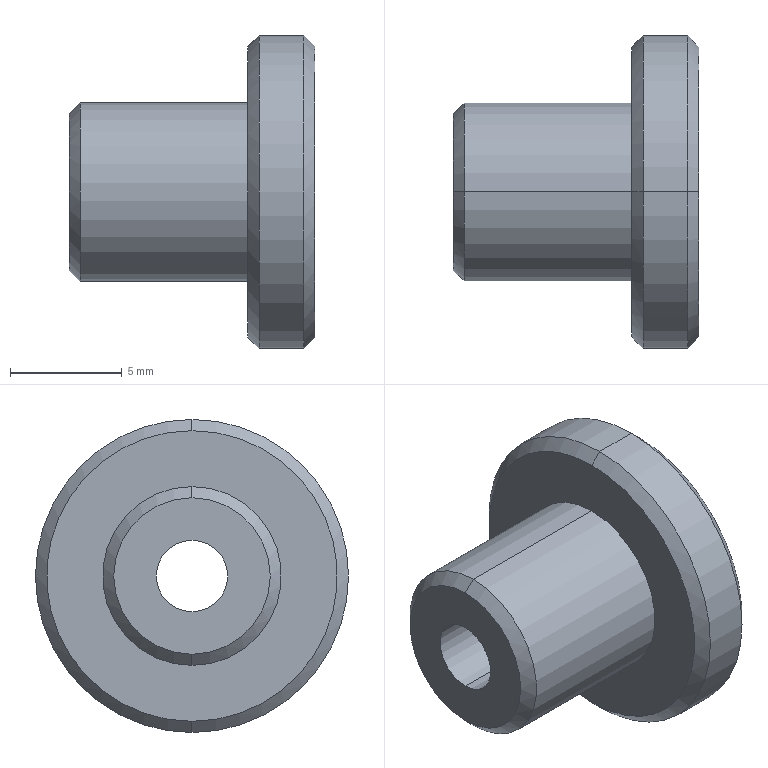Part | SolidWorks | features Chamfer 1, Revolution 1 | 1 solid | 17 faces | box 11 x 14 x 14 mm | volume 760.339 mm3 | cone 8 | cylinder 6 | plane 3 | commonest cylinder face diameters 3.2 x2 8 x2 14 x2
STEP:
#1=CARTESIAN_POINT('',(17.,26.043,1.6));
#2=VERTEX_POINT('',#1);
#3=CARTESIAN_POINT('',(17.,26.043,-1.6));
#4=VERTEX_POINT('',#3);
#5=CARTESIAN_POINT('',(17.,26.043,0.));
#6=DIRECTION('',(1.,0.,0.));
#7=DIRECTION('',(0.,0.,-1.));
#8=AXIS2_PLACEMENT_3D('',#5,#6,#7);
#9=CIRCLE('',#8,1.6);
#10=EDGE_CURVE('',#2,#4,#9,.T.);
#11=ORIENTED_EDGE('',*,*,#10,.F.);
#12=CARTESIAN_POINT('',(17.5,26.043,2.1));
#13=VERTEX_POINT('',#12);
#14=CARTESIAN_POINT('',(17.,26.043,1.6));
#15=DIRECTION('',(0.7071,0.,0.7071));
#16=VECTOR('',#15,1000.);
#17=LINE('',#14,#16);
#18=EDGE_CURVE('',#2,#13,#17,.T.);
#19=ORIENTED_EDGE('',*,*,#18,.T.);
#20=CARTESIAN_POINT('',(17.5,26.043,-2.1));
#21=VERTEX_POINT('',#20);
#22=CARTESIAN_POINT('',(17.5,26.043,0.));
#23=DIRECTION('',(-1.,0.,0.));
#24=DIRECTION('',(0.,0.,-1.));
#25=AXIS2_PLACEMENT_3D('',#22,#23,#24);
#26=CIRCLE('',#25,2.1);
#27=EDGE_CURVE('',#21,#13,#26,.T.);
#28=ORIENTED_EDGE('',*,*,#27,.F.);
#29=CARTESIAN_POINT('',(17.,26.043,-1.6));
#30=DIRECTION('',(0.7071,0.,-0.7071));
#31=VECTOR('',#30,1000.);
#32=LINE('',#29,#31);
#33=EDGE_CURVE('',#4,#21,#32,.T.);
#34=ORIENTED_EDGE('',*,*,#33,.F.);
#35=EDGE_LOOP('',(#11,#19,#28,#34));
#36=FACE_OUTER_BOUND('',#35,.T.);
#37=CARTESIAN_POINT('',(17.,26.043,0.));
#38=DIRECTION('',(1.,0.,0.));
#39=DIRECTION('',(0.,0.,-1.));
#40=AXIS2_PLACEMENT_3D('',#37,#38,#39);
#41=CONICAL_SURFACE('',#40,1.6,0.7854);
#42=ADVANCED_FACE('',(#36),#41,.F.);
#43=CARTESIAN_POINT('',(6.5,26.043,3.5));
#44=VERTEX_POINT('',#43);
#45=CARTESIAN_POINT('',(6.5,26.043,-3.5));
#46=VERTEX_POINT('',#45);
#47=CARTESIAN_POINT('',(6.5,26.043,0.));
#48=DIRECTION('',(-1.,0.,0.));
#49=DIRECTION('',(0.,0.,1.));
#50=AXIS2_PLACEMENT_3D('',#47,#48,#49);
#51=CIRCLE('',#50,3.5);
#52=EDGE_CURVE('',#44,#46,#51,.T.);
#53=ORIENTED_EDGE('',*,*,#52,.F.);
#54=CARTESIAN_POINT('',(7.,26.043,4.));
#55=VERTEX_POINT('',#54);
#56=CARTESIAN_POINT('',(7.,26.043,4.));
#57=DIRECTION('',(0.7071,0.,0.7071));
#58=VECTOR('',#57,1000.);
#59=LINE('',#56,#58);
#60=EDGE_CURVE('',#44,#55,#59,.T.);
#61=ORIENTED_EDGE('',*,*,#60,.T.);
#62=CARTESIAN_POINT('',(7.,26.043,-4.));
#63=VERTEX_POINT('',#62);
#64=CARTESIAN_POINT('',(7.,26.043,0.));
#65=DIRECTION('',(1.,0.,0.));
#66=DIRECTION('',(0.,0.,1.));
#67=AXIS2_PLACEMENT_3D('',#64,#65,#66);
#68=CIRCLE('',#67,4.);
#69=EDGE_CURVE('',#63,#55,#68,.T.);
#70=ORIENTED_EDGE('',*,*,#69,.F.);
#71=CARTESIAN_POINT('',(7.,26.043,-4.));
#72=DIRECTION('',(0.7071,0.,-0.7071));
#73=VECTOR('',#72,1000.);
#74=LINE('',#71,#73);
#75=EDGE_CURVE('',#46,#63,#74,.T.);
#76=ORIENTED_EDGE('',*,*,#75,.F.);
#77=EDGE_LOOP('',(#53,#61,#70,#76));
#78=FACE_OUTER_BOUND('',#77,.T.);
#79=CARTESIAN_POINT('',(7.,26.043,0.));
#80=DIRECTION('',(1.,0.,0.));
#81=DIRECTION('',(0.,0.,-1.));
#82=AXIS2_PLACEMENT_3D('',#79,#80,#81);
#83=CONICAL_SURFACE('',#82,4.,0.7854);
#84=ADVANCED_FACE('',(#78),#83,.T.);
#85=CARTESIAN_POINT('',(17.5,26.043,-6.5));
#86=VERTEX_POINT('',#85);
#87=CARTESIAN_POINT('',(17.5,26.043,6.5));
#88=VERTEX_POINT('',#87);
#89=CARTESIAN_POINT('',(17.5,26.043,0.));
#90=DIRECTION('',(1.,0.,0.));
#91=DIRECTION('',(0.,0.,-1.));
#92=AXIS2_PLACEMENT_3D('',#89,#90,#91);
#93=CIRCLE('',#92,6.5);
#94=EDGE_CURVE('',#86,#88,#93,.T.);
#95=ORIENTED_EDGE('',*,*,#94,.F.);
#96=CARTESIAN_POINT('',(17.,26.043,-7.));
#97=VERTEX_POINT('',#96);
#98=CARTESIAN_POINT('',(17.5,26.043,-6.5));
#99=DIRECTION('',(-0.7071,0.,-0.7071));
#100=VECTOR('',#99,1000.);
#101=LINE('',#98,#100);
#102=EDGE_CURVE('',#86,#97,#101,.T.);
#103=ORIENTED_EDGE('',*,*,#102,.T.);
#104=CARTESIAN_POINT('',(17.,26.043,7.));
#105=VERTEX_POINT('',#104);
#106=CARTESIAN_POINT('',(17.,26.043,0.));
#107=DIRECTION('',(-1.,0.,0.));
#108=DIRECTION('',(0.,0.,-1.));
#109=AXIS2_PLACEMENT_3D('',#106,#107,#108);
#110=CIRCLE('',#109,7.);
#111=EDGE_CURVE('',#105,#97,#110,.T.);
#112=ORIENTED_EDGE('',*,*,#111,.F.);
#113=CARTESIAN_POINT('',(17.5,26.043,6.5));
#114=DIRECTION('',(-0.7071,0.,0.7071));
#115=VECTOR('',#114,1000.);
#116=LINE('',#113,#115);
#117=EDGE_CURVE('',#88,#105,#116,.T.);
#118=ORIENTED_EDGE('',*,*,#117,.F.);
#119=EDGE_LOOP('',(#95,#103,#112,#118));
#120=FACE_OUTER_BOUND('',#119,.T.);
#121=CARTESIAN_POINT('',(17.5,26.043,0.));
#122=DIRECTION('',(-1.,0.,0.));
#123=DIRECTION('',(0.,0.,1.));
#124=AXIS2_PLACEMENT_3D('',#121,#122,#123);
#125=CONICAL_SURFACE('',#124,6.5,0.7854);
#126=ADVANCED_FACE('',(#120),#125,.T.);
#127=CARTESIAN_POINT('',(14.5,26.043,6.5));
#128=VERTEX_POINT('',#127);
#129=CARTESIAN_POINT('',(14.5,26.043,-6.5));
#130=VERTEX_POINT('',#129);
#131=CARTESIAN_POINT('',(14.5,26.043,0.));
#132=DIRECTION('',(-1.,0.,0.));
#133=DIRECTION('',(0.,0.,1.));
#134=AXIS2_PLACEMENT_3D('',#131,#132,#133);
#135=CIRCLE('',#134,6.5);
#136=EDGE_CURVE('',#128,#130,#135,.T.);
#137=ORIENTED_EDGE('',*,*,#136,.F.);
#138=CARTESIAN_POINT('',(15.,26.043,7.));
#139=VERTEX_POINT('',#138);
#140=CARTESIAN_POINT('',(15.,26.043,7.));
#141=DIRECTION('',(0.7071,0.,0.7071));
#142=VECTOR('',#141,1000.);
#143=LINE('',#140,#142);
#144=EDGE_CURVE('',#128,#139,#143,.T.);
#145=ORIENTED_EDGE('',*,*,#144,.T.);
#146=CARTESIAN_POINT('',(15.,26.043,-7.));
#147=VERTEX_POINT('',#146);
#148=CARTESIAN_POINT('',(15.,26.043,0.));
#149=DIRECTION('',(1.,0.,0.));
#150=DIRECTION('',(0.,0.,1.));
#151=AXIS2_PLACEMENT_3D('',#148,#149,#150);
#152=CIRCLE('',#151,7.);
#153=EDGE_CURVE('',#147,#139,#152,.T.);
#154=ORIENTED_EDGE('',*,*,#153,.F.);
#155=CARTESIAN_POINT('',(15.,26.043,-7.));
#156=DIRECTION('',(0.7071,0.,-0.7071));
#157=VECTOR('',#156,1000.);
#158=LINE('',#155,#157);
#159=EDGE_CURVE('',#130,#147,#158,.T.);
#160=ORIENTED_EDGE('',*,*,#159,.F.);
#161=EDGE_LOOP('',(#137,#145,#154,#160));
#162=FACE_OUTER_BOUND('',#161,.T.);
#163=CARTESIAN_POINT('',(15.,26.043,0.));
#164=DIRECTION('',(1.,0.,0.));
#165=DIRECTION('',(0.,0.,-1.));
#166=AXIS2_PLACEMENT_3D('',#163,#164,#165);
#167=CONICAL_SURFACE('',#166,7.,0.7854);
#168=ADVANCED_FACE('',(#162),#167,.T.);
#169=ORIENTED_EDGE('',*,*,#153,.T.);
#170=CARTESIAN_POINT('',(17.5,26.043,7.));
#171=DIRECTION('',(1.,0.,0.));
#172=VECTOR('',#171,1000.);
#173=LINE('',#170,#172);
#174=EDGE_CURVE('',#139,#105,#173,.T.);
#175=ORIENTED_EDGE('',*,*,#174,.T.);
#176=ORIENTED_EDGE('',*,*,#111,.T.);
#177=CARTESIAN_POINT('',(17.5,26.043,-7.));
#178=DIRECTION('',(1.,0.,0.));
#179=VECTOR('',#178,1000.);
#180=LINE('',#177,#179);
#181=EDGE_CURVE('',#147,#97,#180,.T.);
#182=ORIENTED_EDGE('',*,*,#181,.F.);
#183=EDGE_LOOP('',(#169,#175,#176,#182));
#184=FACE_OUTER_BOUND('',#183,.T.);
#185=CARTESIAN_POINT('',(17.5,26.043,0.));
#186=DIRECTION('',(1.,0.,0.));
#187=DIRECTION('',(0.,0.,-1.));
#188=AXIS2_PLACEMENT_3D('',#185,#186,#187);
#189=CYLINDRICAL_SURFACE('',#188,7.);
#190=ADVANCED_FACE('',(#184),#189,.T.);
#191=ORIENTED_EDGE('',*,*,#69,.T.);
#192=CARTESIAN_POINT('',(14.5,26.043,4.));
#193=VERTEX_POINT('',#192);
#194=CARTESIAN_POINT('',(17.5,26.043,4.));
#195=DIRECTION('',(1.,0.,0.));
#196=VECTOR('',#195,1000.);
#197=LINE('',#194,#196);
#198=EDGE_CURVE('',#55,#193,#197,.T.);
#199=ORIENTED_EDGE('',*,*,#198,.T.);
#200=CARTESIAN_POINT('',(14.5,26.043,-4.));
#201=VERTEX_POINT('',#200);
#202=CARTESIAN_POINT('',(14.5,26.043,0.));
#203=DIRECTION('',(1.,0.,0.));
#204=DIRECTION('',(0.,0.,-1.));
#205=AXIS2_PLACEMENT_3D('',#202,#203,#204);
#206=CIRCLE('',#205,4.);
#207=EDGE_CURVE('',#201,#193,#206,.T.);
#208=ORIENTED_EDGE('',*,*,#207,.F.);
#209=CARTESIAN_POINT('',(17.5,26.043,-4.));
#210=DIRECTION('',(1.,0.,0.));
#211=VECTOR('',#210,1000.);
#212=LINE('',#209,#211);
#213=EDGE_CURVE('',#63,#201,#212,.T.);
#214=ORIENTED_EDGE('',*,*,#213,.F.);
#215=EDGE_LOOP('',(#191,#199,#208,#214));
#216=FACE_OUTER_BOUND('',#215,.T.);
#217=CARTESIAN_POINT('',(17.5,26.043,0.));
#218=DIRECTION('',(1.,0.,0.));
#219=DIRECTION('',(0.,0.,-1.));
#220=AXIS2_PLACEMENT_3D('',#217,#218,#219);
#221=CYLINDRICAL_SURFACE('',#220,4.);
#222=ADVANCED_FACE('',(#216),#221,.T.);
#223=CARTESIAN_POINT('',(6.5,26.043,1.6));
#224=VERTEX_POINT('',#223);
#225=CARTESIAN_POINT('',(6.5,26.043,-1.6));
#226=VERTEX_POINT('',#225);
#227=CARTESIAN_POINT('',(6.5,26.043,0.));
#228=DIRECTION('',(1.,0.,0.));
#229=DIRECTION('',(0.,0.,-1.));
#230=AXIS2_PLACEMENT_3D('',#227,#228,#229);
#231=CIRCLE('',#230,1.6);
#232=EDGE_CURVE('',#224,#226,#231,.T.);
#233=ORIENTED_EDGE('',*,*,#232,.F.);
#234=CARTESIAN_POINT('',(17.5,26.043,1.6));
#235=DIRECTION('',(1.,0.,0.));
#236=VECTOR('',#235,1000.);
#237=LINE('',#234,#236);
#238=EDGE_CURVE('',#224,#2,#237,.T.);
#239=ORIENTED_EDGE('',*,*,#238,.T.);
#240=ORIENTED_EDGE('',*,*,#10,.T.);
#241=CARTESIAN_POINT('',(17.5,26.043,-1.6));
#242=DIRECTION('',(1.,0.,0.));
#243=VECTOR('',#242,1000.);
#244=LINE('',#241,#243);
#245=EDGE_CURVE('',#226,#4,#244,.T.);
#246=ORIENTED_EDGE('',*,*,#245,.F.);
#247=EDGE_LOOP('',(#233,#239,#240,#246));
#248=FACE_OUTER_BOUND('',#247,.T.);
#249=CARTESIAN_POINT('',(17.5,26.043,0.));
#250=DIRECTION('',(1.,0.,0.));
#251=DIRECTION('',(0.,0.,-1.));
#252=AXIS2_PLACEMENT_3D('',#249,#250,#251);
#253=CYLINDRICAL_SURFACE('',#252,1.6);
#254=ADVANCED_FACE('',(#248),#253,.F.);
#255=CARTESIAN_POINT('',(17.5,26.043,0.));
#256=DIRECTION('',(1.,0.,0.));
#257=DIRECTION('',(0.,0.,-1.));
#258=AXIS2_PLACEMENT_3D('',#255,#256,#257);
#259=CIRCLE('',#258,6.5);
#260=EDGE_CURVE('',#88,#86,#259,.T.);
#261=ORIENTED_EDGE('',*,*,#260,.T.);
#262=ORIENTED_EDGE('',*,*,#94,.T.);
#263=EDGE_LOOP('',(#261,#262));
#264=FACE_OUTER_BOUND('',#263,.T.);
#265=ORIENTED_EDGE('',*,*,#27,.T.);
#266=CARTESIAN_POINT('',(17.5,26.043,0.));
#267=DIRECTION('',(-1.,0.,0.));
#268=DIRECTION('',(0.,0.,-1.));
#269=AXIS2_PLACEMENT_3D('',#266,#267,#268);
#270=CIRCLE('',#269,2.1);
#271=EDGE_CURVE('',#13,#21,#270,.T.);
#272=ORIENTED_EDGE('',*,*,#271,.T.);
#273=EDGE_LOOP('',(#265,#272));
#274=FACE_BOUND('',#273,.T.);
#275=CARTESIAN_POINT('',(17.5,33.043,0.));
#276=DIRECTION('',(1.,0.,0.));
#277=DIRECTION('',(0.,0.,-1.));
#278=AXIS2_PLACEMENT_3D('',#275,#276,#277);
#279=PLANE('',#278);
#280=ADVANCED_FACE('',(#264,#274),#279,.T.);
#281=ORIENTED_EDGE('',*,*,#238,.F.);
#282=CARTESIAN_POINT('',(6.5,26.043,0.));
#283=DIRECTION('',(1.,0.,0.));
#284=DIRECTION('',(0.,0.,-1.));
#285=AXIS2_PLACEMENT_3D('',#282,#283,#284);
#286=CIRCLE('',#285,1.6);
#287=EDGE_CURVE('',#226,#224,#286,.T.);
#288=ORIENTED_EDGE('',*,*,#287,.F.);
#289=ORIENTED_EDGE('',*,*,#245,.T.);
#290=CARTESIAN_POINT('',(17.,26.043,0.));
#291=DIRECTION('',(1.,0.,0.));
#292=DIRECTION('',(0.,0.,-1.));
#293=AXIS2_PLACEMENT_3D('',#290,#291,#292);
#294=CIRCLE('',#293,1.6);
#295=EDGE_CURVE('',#4,#2,#294,.T.);
#296=ORIENTED_EDGE('',*,*,#295,.T.);
#297=EDGE_LOOP('',(#281,#288,#289,#296));
#298=FACE_OUTER_BOUND('',#297,.T.);
#299=CARTESIAN_POINT('',(17.5,26.043,0.));
#300=DIRECTION('',(1.,0.,0.));
#301=DIRECTION('',(0.,0.,-1.));
#302=AXIS2_PLACEMENT_3D('',#299,#300,#301);
#303=CYLINDRICAL_SURFACE('',#302,1.6);
#304=ADVANCED_FACE('',(#298),#303,.F.);
#305=CARTESIAN_POINT('',(6.5,26.043,0.));
#306=DIRECTION('',(-1.,0.,0.));
#307=DIRECTION('',(0.,0.,1.));
#308=AXIS2_PLACEMENT_3D('',#305,#306,#307);
#309=CIRCLE('',#308,3.5);
#310=EDGE_CURVE('',#46,#44,#309,.T.);
#311=ORIENTED_EDGE('',*,*,#310,.T.);
#312=ORIENTED_EDGE('',*,*,#52,.T.);
#313=EDGE_LOOP('',(#311,#312));
#314=FACE_OUTER_BOUND('',#313,.T.);
#315=ORIENTED_EDGE('',*,*,#287,.T.);
#316=ORIENTED_EDGE('',*,*,#232,.T.);
#317=EDGE_LOOP('',(#315,#316));
#318=FACE_BOUND('',#317,.T.);
#319=CARTESIAN_POINT('',(6.5,30.043,0.));
#320=DIRECTION('',(-1.,0.,0.));
#321=DIRECTION('',(0.,0.,1.));
#322=AXIS2_PLACEMENT_3D('',#319,#320,#321);
#323=PLANE('',#322);
#324=ADVANCED_FACE('',(#314,#318),#323,.T.);
#325=ORIENTED_EDGE('',*,*,#198,.F.);
#326=CARTESIAN_POINT('',(7.,26.043,0.));
#327=DIRECTION('',(1.,0.,0.));
#328=DIRECTION('',(0.,0.,1.));
#329=AXIS2_PLACEMENT_3D('',#326,#327,#328);
#330=CIRCLE('',#329,4.);
#331=EDGE_CURVE('',#55,#63,#330,.T.);
#332=ORIENTED_EDGE('',*,*,#331,.T.);
#333=ORIENTED_EDGE('',*,*,#213,.T.);
#334=CARTESIAN_POINT('',(14.5,26.043,0.));
#335=DIRECTION('',(1.,0.,0.));
#336=DIRECTION('',(0.,0.,-1.));
#337=AXIS2_PLACEMENT_3D('',#334,#335,#336);
#338=CIRCLE('',#337,4.);
#339=EDGE_CURVE('',#193,#201,#338,.T.);
#340=ORIENTED_EDGE('',*,*,#339,.F.);
#341=EDGE_LOOP('',(#325,#332,#333,#340));
#342=FACE_OUTER_BOUND('',#341,.T.);
#343=CARTESIAN_POINT('',(17.5,26.043,0.));
#344=DIRECTION('',(1.,0.,0.));
#345=DIRECTION('',(0.,0.,-1.));
#346=AXIS2_PLACEMENT_3D('',#343,#344,#345);
#347=CYLINDRICAL_SURFACE('',#346,4.);
#348=ADVANCED_FACE('',(#342),#347,.T.);
#349=CARTESIAN_POINT('',(14.5,26.043,0.));
#350=DIRECTION('',(-1.,0.,0.));
#351=DIRECTION('',(0.,0.,1.));
#352=AXIS2_PLACEMENT_3D('',#349,#350,#351);
#353=CIRCLE('',#352,6.5);
#354=EDGE_CURVE('',#130,#128,#353,.T.);
#355=ORIENTED_EDGE('',*,*,#354,.T.);
#356=ORIENTED_EDGE('',*,*,#136,.T.);
#357=EDGE_LOOP('',(#355,#356));
#358=FACE_OUTER_BOUND('',#357,.T.);
#359=ORIENTED_EDGE('',*,*,#207,.T.);
#360=ORIENTED_EDGE('',*,*,#339,.T.);
#361=EDGE_LOOP('',(#359,#360));
#362=FACE_BOUND('',#361,.T.);
#363=CARTESIAN_POINT('',(14.5,30.043,0.));
#364=DIRECTION('',(-1.,0.,0.));
#365=DIRECTION('',(0.,0.,1.));
#366=AXIS2_PLACEMENT_3D('',#363,#364,#365);
#367=PLANE('',#366);
#368=ADVANCED_FACE('',(#358,#362),#367,.T.);
#369=ORIENTED_EDGE('',*,*,#174,.F.);
#370=CARTESIAN_POINT('',(15.,26.043,0.));
#371=DIRECTION('',(1.,0.,0.));
#372=DIRECTION('',(0.,0.,1.));
#373=AXIS2_PLACEMENT_3D('',#370,#371,#372);
#374=CIRCLE('',#373,7.);
#375=EDGE_CURVE('',#139,#147,#374,.T.);
#376=ORIENTED_EDGE('',*,*,#375,.T.);
#377=ORIENTED_EDGE('',*,*,#181,.T.);
#378=CARTESIAN_POINT('',(17.,26.043,0.));
#379=DIRECTION('',(-1.,0.,0.));
#380=DIRECTION('',(0.,0.,-1.));
#381=AXIS2_PLACEMENT_3D('',#378,#379,#380);
#382=CIRCLE('',#381,7.);
#383=EDGE_CURVE('',#97,#105,#382,.T.);
#384=ORIENTED_EDGE('',*,*,#383,.T.);
#385=EDGE_LOOP('',(#369,#376,#377,#384));
#386=FACE_OUTER_BOUND('',#385,.T.);
#387=CARTESIAN_POINT('',(17.5,26.043,0.));
#388=DIRECTION('',(1.,0.,0.));
#389=DIRECTION('',(0.,0.,-1.));
#390=AXIS2_PLACEMENT_3D('',#387,#388,#389);
#391=CYLINDRICAL_SURFACE('',#390,7.);
#392=ADVANCED_FACE('',(#386),#391,.T.);
#393=ORIENTED_EDGE('',*,*,#144,.F.);
#394=ORIENTED_EDGE('',*,*,#354,.F.);
#395=ORIENTED_EDGE('',*,*,#159,.T.);
#396=ORIENTED_EDGE('',*,*,#375,.F.);
#397=EDGE_LOOP('',(#393,#394,#395,#396));
#398=FACE_OUTER_BOUND('',#397,.T.);
#399=CARTESIAN_POINT('',(15.,26.043,0.));
#400=DIRECTION('',(1.,0.,0.));
#401=DIRECTION('',(0.,0.,-1.));
#402=AXIS2_PLACEMENT_3D('',#399,#400,#401);
#403=CONICAL_SURFACE('',#402,7.,0.7854);
#404=ADVANCED_FACE('',(#398),#403,.T.);
#405=ORIENTED_EDGE('',*,*,#102,.F.);
#406=ORIENTED_EDGE('',*,*,#260,.F.);
#407=ORIENTED_EDGE('',*,*,#117,.T.);
#408=ORIENTED_EDGE('',*,*,#383,.F.);
#409=EDGE_LOOP('',(#405,#406,#407,#408));
#410=FACE_OUTER_BOUND('',#409,.T.);
#411=CARTESIAN_POINT('',(17.5,26.043,0.));
#412=DIRECTION('',(-1.,0.,0.));
#413=DIRECTION('',(0.,0.,1.));
#414=AXIS2_PLACEMENT_3D('',#411,#412,#413);
#415=CONICAL_SURFACE('',#414,6.5,0.7854);
#416=ADVANCED_FACE('',(#410),#415,.T.);
#417=ORIENTED_EDGE('',*,*,#60,.F.);
#418=ORIENTED_EDGE('',*,*,#310,.F.);
#419=ORIENTED_EDGE('',*,*,#75,.T.);
#420=ORIENTED_EDGE('',*,*,#331,.F.);
#421=EDGE_LOOP('',(#417,#418,#419,#420));
#422=FACE_OUTER_BOUND('',#421,.T.);
#423=CARTESIAN_POINT('',(7.,26.043,0.));
#424=DIRECTION('',(1.,0.,0.));
#425=DIRECTION('',(0.,0.,-1.));
#426=AXIS2_PLACEMENT_3D('',#423,#424,#425);
#427=CONICAL_SURFACE('',#426,4.,0.7854);
#428=ADVANCED_FACE('',(#422),#427,.T.);
#429=ORIENTED_EDGE('',*,*,#18,.F.);
#430=ORIENTED_EDGE('',*,*,#295,.F.);
#431=ORIENTED_EDGE('',*,*,#33,.T.);
#432=ORIENTED_EDGE('',*,*,#271,.F.);
#433=EDGE_LOOP('',(#429,#430,#431,#432));
#434=FACE_OUTER_BOUND('',#433,.T.);
#435=CARTESIAN_POINT('',(17.,26.043,0.));
#436=DIRECTION('',(1.,0.,0.));
#437=DIRECTION('',(0.,0.,-1.));
#438=AXIS2_PLACEMENT_3D('',#435,#436,#437);
#439=CONICAL_SURFACE('',#438,1.6,0.7854);
#440=ADVANCED_FACE('',(#434),#439,.F.);
#441=CLOSED_SHELL('',(#42,#84,#126,#168,#190,#222,#254,#280,#304,#324,#348,#368,#392,#404,#416,#428,#440));
#442=MANIFOLD_SOLID_BREP('',#441);
#443=CARTESIAN_POINT('',(0.,0.,0.));
#444=DIRECTION('',(0.,0.,1.));
#445=DIRECTION('',(1.,0.,0.));
#446=AXIS2_PLACEMENT_3D('',#443,#444,#445);
#447=(LENGTH_UNIT()NAMED_UNIT(*)SI_UNIT(.MILLI.,.METRE.));
#448=UNCERTAINTY_MEASURE_WITH_UNIT(LENGTH_MEASURE(0.00001),#447,'','');
#449=(NAMED_UNIT(*)PLANE_ANGLE_UNIT()SI_UNIT($,.RADIAN.));
#450=(NAMED_UNIT(*)SI_UNIT($,.STERADIAN.)SOLID_ANGLE_UNIT());
#451=(GEOMETRIC_REPRESENTATION_CONTEXT(3)GLOBAL_UNCERTAINTY_ASSIGNED_CONTEXT((#448))GLOBAL_UNIT_ASSIGNED_CONTEXT((#447,#449,#450))REPRESENTATION_CONTEXT('',''));
#452=ADVANCED_BREP_SHAPE_REPRESENTATION('',(#442,#446),#451);